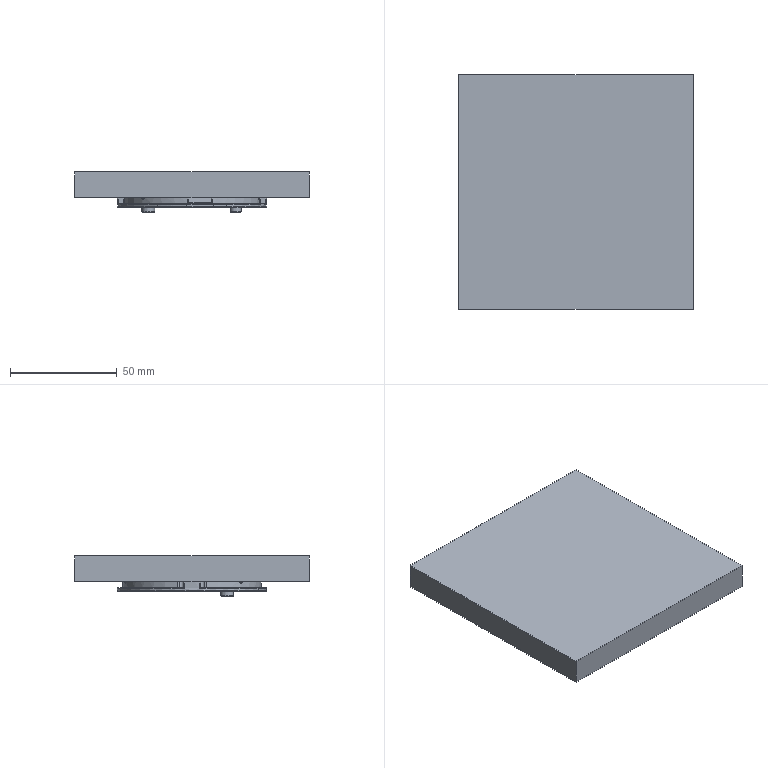NC program | NX | posted with a generic post | part box 110 x 110 x 18.8 mm
Lines 7252 to 9086 of 9447, first 1548 of 1823 lines:
(CAVITY_MILL_COPY_1_COPY_COPY , TOOL : D2)
N14466 T02 M6
N14468 G54
N14470 G17 G0 G90 X19.668 Y-21.389 S9500 M3
N14472 G43 Z30. H2
N14474 Z-4.143
N14476 G94 G1 Z-5.143 F1000.
N14478 X20.63 Y-20.963
N14480 G3 X20.925 Y-20.56 R0.5
N14482 X20.616 Y-20. R0.557
N14484 G1 X20.071
N14486 G3 X19.271 Y-20.4 R1.
N14488 G1 Z-4.143
N14490 G0 Z30.
N14492 X14.4 Y-21.675
N14494 Z-10.625
N14496 G1 Z-11.625
N14498 G3 X14.825 Y-20.857 R1.
N14500 G1 Y-20.
N14502 X13.968
N14504 G3 X13.168 Y-20.4 R1.
N14506 G1 Z-10.625
N14508 G0 X14.325 Y-21.675 Z-10.75
N14510 G1 Z-11.75
N14512 G3 X14.75 Y-20.857 R1.
N14514 G1 Y-20.
N14516 X13.893
N14518 G3 X13.093 Y-20.4 R1.
N14520 G1 Z-10.75
N14522 G0 X14.325 Y-21.675 Z-10.875
N14524 G1 Z-11.875
N14526 G3 X14.75 Y-20.857 R1.
N14528 G1 Y-20.
N14530 X13.893
N14532 G3 X13.093 Y-20.4 R1.
N14534 G1 Z-10.875
N14536 G0 X14.325 Y-21.675 Z-11.
N14538 G1 Z-12.
N14540 G3 X14.75 Y-20.857 R1.
N14542 G1 Y-20.
N14544 X13.893
N14546 G3 X13.093 Y-20.4 R1.
N14548 G1 Z-11.
N14550 G0 Z30.
N14552 X24.9 Y-13.399
N14554 Z-4.143
N14556 G1 Z-5.143
N14558 G3 X24.5 Y-14.199 R1.
N14560 G1 Y-14.744
N14562 G3 X25.06 Y-15.053 R0.557
N14564 X25.463 Y-14.758 R0.5
N14566 G1 X25.301 Y-14.289
N14568 Z-4.143
N14570 G0 Z30.
N14572 X33.412 Y-4.088
N14574 Z-4.143
N14576 G1 Z-5.143
N14578 G3 X32.74 Y-4.451 R1.
N14580 G2 X32.126 Y-4.949 R1.943
N14582 G1 X32.092 Y-4.97
N14584 X32.086 Y-5.011
N14586 X32.112 Y-5.04
N14588 G2 X32.545 Y-5.702 R1.943
N14590 G3 X33.075 Y-6.251 R1.
N14592 G1 Z-4.143
N14594 G0 X33.471 Y-4.092 Z-4.286
N14596 G1 Z-5.286
N14598 G3 X32.802 Y-4.465 R1.
N14600 G2 X32.18 Y-4.986 R2.
N14602 G1 X32.152 Y-5.
N14604 G2 X32.609 Y-5.708 R2.
N14606 G3 X33.133 Y-6.266 R1.
N14608 G1 Z-4.286
N14610 G0 X33.471 Y-4.092 Z-4.429
N14612 G1 Z-5.429
N14614 G3 X32.802 Y-4.465 R1.
N14616 G2 X32.18 Y-4.986 R2.
N14618 G1 X32.152 Y-5.
N14620 G2 X32.609 Y-5.708 R2.
N14622 G3 X33.133 Y-6.266 R1.
N14624 G1 Z-4.429
N14626 G0 X33.471 Y-4.092 Z-4.571
N14628 G1 Z-5.571
N14630 G3 X32.802 Y-4.465 R1.
N14632 G2 X32.18 Y-4.986 R2.
N14634 G1 X32.152 Y-5.
N14636 G2 X32.609 Y-5.708 R2.
N14638 G3 X33.133 Y-6.266 R1.
N14640 G1 Z-4.571
N14642 G0 X33.471 Y-4.092 Z-4.714
N14644 G1 Z-5.714
N14646 G3 X32.802 Y-4.465 R1.
N14648 G2 X32.18 Y-4.986 R2.
N14650 G1 X32.152 Y-5.
N14652 G2 X32.609 Y-5.708 R2.
N14654 G3 X33.133 Y-6.266 R1.
N14656 G1 Z-4.714
N14658 G0 X33.471 Y-4.092 Z-4.857
N14660 G1 Z-5.857
N14662 G3 X32.802 Y-4.465 R1.
N14664 G2 X32.18 Y-4.986 R2.
N14666 G1 X32.152 Y-5.
N14668 G2 X32.609 Y-5.708 R2.
N14670 G3 X33.133 Y-6.266 R1.
N14672 G1 Z-4.857
N14674 G0 X33.471 Y-4.092 Z-5.
N14676 G1 Z-6.
N14678 G3 X32.802 Y-4.465 R1.
N14680 G2 X32.18 Y-4.986 R2.
N14682 G1 X32.152 Y-5.
N14684 G2 X32.609 Y-5.708 R2.
N14686 G3 X33.133 Y-6.266 R1.
N14688 G1 Z-5.
N14690 G0 X33.471 Y-4.092 Z-5.15
N14692 G1 Z-6.15
N14694 G3 X32.802 Y-4.465 R1.
N14696 G2 X32.18 Y-4.986 R2.
N14698 G1 X32.152 Y-5.
N14700 G2 X32.609 Y-5.708 R2.
N14702 G3 X33.133 Y-6.266 R1.
N14704 G1 Z-5.15
N14706 G0 X33.471 Y-4.092 Z-5.3
N14708 G1 Z-6.3
N14710 G3 X32.802 Y-4.465 R1.
N14712 G2 X32.18 Y-4.986 R2.
N14714 G1 X32.152 Y-5.
N14716 G2 X32.609 Y-5.708 R2.
N14718 G3 X33.133 Y-6.266 R1.
N14720 G1 Z-5.3
N14722 G0 X33.471 Y-4.092 Z-5.45
N14724 G1 Z-6.45
N14726 G3 X32.802 Y-4.465 R1.
N14728 G2 X32.18 Y-4.986 R2.
N14730 G1 X32.152 Y-5.
N14732 G2 X32.609 Y-5.708 R2.
N14734 G3 X33.133 Y-6.266 R1.
N14736 G1 Z-5.45
N14738 G0 X33.471 Y-4.092 Z-5.6
N14740 G1 Z-6.6
N14742 G3 X32.802 Y-4.465 R1.
N14744 G2 X32.18 Y-4.986 R2.
N14746 G1 X32.152 Y-5.
N14748 G2 X32.609 Y-5.708 R2.
N14750 G3 X33.133 Y-6.266 R1.
N14752 G1 Z-5.6
N14754 G0 X33.471 Y-4.092 Z-5.75
N14756 G1 Z-6.75
N14758 G3 X32.802 Y-4.465 R1.
N14760 G2 X32.18 Y-4.986 R2.
N14762 G1 X32.152 Y-5.
N14764 G2 X32.609 Y-5.708 R2.
N14766 G3 X33.133 Y-6.266 R1.
N14768 G1 Z-5.75
N14770 G0 X33.471 Y-4.092 Z-5.9
N14772 G1 Z-6.9
N14774 G3 X32.802 Y-4.465 R1.
N14776 G2 X32.18 Y-4.986 R2.
N14778 G1 X32.152 Y-5.
N14780 G2 X32.609 Y-5.708 R2.
N14782 G3 X33.133 Y-6.266 R1.
N14784 G1 Z-5.9
N14786 G0 X33.471 Y-4.092 Z-6.05
N14788 G1 Z-7.05
N14790 G3 X32.802 Y-4.465 R1.
N14792 G2 X32.18 Y-4.986 R2.
N14794 G1 X32.152 Y-5.
N14796 G2 X32.609 Y-5.708 R2.
N14798 G3 X33.133 Y-6.266 R1.
N14800 G1 Z-6.05
N14802 G0 X33.471 Y-4.092 Z-6.2
N14804 G1 Z-7.2
N14806 G3 X32.802 Y-4.465 R1.
N14808 G2 X32.18 Y-4.986 R2.
N14810 G1 X32.152 Y-5.
N14812 G2 X32.609 Y-5.708 R2.
N14814 G3 X33.133 Y-6.266 R1.
N14816 G1 Z-6.2
N14818 G0 X33.471 Y-4.092 Z-6.35
N14820 G1 Z-7.35
N14822 G3 X32.802 Y-4.465 R1.
N14824 G2 X32.18 Y-4.986 R2.
N14826 G1 X32.152 Y-5.
N14828 G2 X32.609 Y-5.708 R2.
N14830 G3 X33.133 Y-6.266 R1.
N14832 G1 Z-6.35
N14834 G0 X33.471 Y-4.092 Z-6.5
N14836 G1 Z-7.5
N14838 G3 X32.802 Y-4.465 R1.
N14840 G2 X32.18 Y-4.986 R2.
N14842 G1 X32.152 Y-5.
N14844 G2 X32.609 Y-5.708 R2.
N14846 G3 X33.133 Y-6.266 R1.
N14848 G1 Z-6.5
N14850 G0 X33.471 Y-4.092 Z-6.65
N14852 G1 Z-7.65
N14854 G3 X32.802 Y-4.465 R1.
N14856 G2 X32.18 Y-4.986 R2.
N14858 G1 X32.152 Y-5.
N14860 G2 X32.609 Y-5.708 R2.
N14862 G3 X33.133 Y-6.266 R1.
N14864 G1 Z-6.65
N14866 G0 X33.471 Y-4.092 Z-6.8
N14868 G1 Z-7.8
N14870 G3 X32.802 Y-4.465 R1.
N14872 G2 X32.18 Y-4.986 R2.
N14874 G1 X32.152 Y-5.
N14876 G2 X32.609 Y-5.708 R2.
N14878 G3 X33.133 Y-6.266 R1.
N14880 G1 Z-6.8
N14882 G0 X33.471 Y-4.092 Z-6.95
N14884 G1 Z-7.95
N14886 G3 X32.802 Y-4.465 R1.
N14888 G2 X32.18 Y-4.986 R2.
N14890 G1 X32.152 Y-5.
N14892 G2 X32.609 Y-5.708 R2.
N14894 G3 X33.133 Y-6.266 R1.
N14896 G1 Z-6.95
N14898 G0 X33.471 Y-4.092 Z-7.1
N14900 G1 Z-8.1
N14902 G3 X32.802 Y-4.465 R1.
N14904 G2 X32.18 Y-4.986 R2.
N14906 G1 X32.152 Y-5.
N14908 G2 X32.609 Y-5.708 R2.
N14910 G3 X33.133 Y-6.266 R1.
N14912 G1 Z-7.1
N14914 G0 X33.471 Y-4.092 Z-7.25
N14916 G1 Z-8.25
N14918 G3 X32.802 Y-4.465 R1.
N14920 G2 X32.188 Y-4.981 R2.
N14922 G1 X32.152 Y-5.
N14924 G2 X32.609 Y-5.708 R2.
N14926 G3 X33.133 Y-6.266 R1.
N14928 G1 Z-7.25
N14930 G0 X33.471 Y-4.092 Z-7.4
N14932 G1 Z-8.4
N14934 G3 X32.802 Y-4.465 R1.
N14936 G2 X32.188 Y-4.981 R2.
N14938 G1 X32.152 Y-5.
N14940 G2 X32.609 Y-5.708 R2.
N14942 G3 X33.133 Y-6.266 R1.
N14944 G1 Z-7.4
N14946 G0 X33.471 Y-4.092 Z-7.55
N14948 G1 Z-8.55
N14950 G3 X32.802 Y-4.465 R1.
N14952 G2 X32.188 Y-4.981 R2.
N14954 G1 X32.152 Y-5.
N14956 G2 X32.609 Y-5.708 R2.
N14958 G3 X33.133 Y-6.266 R1.
N14960 G1 Z-7.55
N14962 G0 X33.471 Y-4.092 Z-7.7
N14964 G1 Z-8.7
N14966 G3 X32.802 Y-4.465 R1.
N14968 G2 X32.188 Y-4.981 R2.
N14970 G1 X32.152 Y-5.
N14972 G2 X32.609 Y-5.708 R2.
N14974 G3 X33.133 Y-6.266 R1.
N14976 G1 Z-7.7
N14978 G0 X33.471 Y-4.092 Z-7.85
N14980 G1 Z-8.85
N14982 G3 X32.802 Y-4.465 R1.
N14984 G2 X32.188 Y-4.981 R2.
N14986 G1 X32.152 Y-5.
N14988 G2 X32.609 Y-5.708 R2.
N14990 G3 X33.133 Y-6.266 R1.
N14992 G1 Z-7.85
N14994 G0 X33.471 Y-4.092 Z-8.
N14996 G1 Z-9.
N14998 G3 X32.802 Y-4.465 R1.
N15000 G2 X32.188 Y-4.981 R2.
N15002 G1 X32.152 Y-5.
N15004 G2 X32.609 Y-5.708 R2.
N15006 G3 X33.133 Y-6.266 R1.
N15008 G1 Z-8.
N15010 G0 X34.2 Y-5.347 Z-8.147
N15012 G1 Z-9.147
N15014 G3 X33.4 Y-4.947 R1.
N15016 G1 X32.248
N15018 X32.188 Y-4.981
N15020 X32.152 Y-5.
N15022 G2 X32.694 Y-5.996 R2.
N15024 G3 X33.128 Y-6.627 R1.
N15026 G1 Z-8.147
N15028 G0 X34.222 Y-5.4 Z-8.294
N15030 G1 Z-9.294
N15032 G3 X33.422 Y-5. R1.
N15034 G1 X32.198
N15036 X32.152
N15038 G2 X32.703 Y-6.041 R2.
N15040 G3 X33.123 Y-6.682 R1.
N15042 G1 Z-8.294
N15044 G0 X34.222 Y-5.4 Z-8.441
N15046 G1 Z-9.441
N15048 G3 X33.422 Y-5. R1.
N15050 G1 X32.198
N15052 X32.152
N15054 G2 X32.703 Y-6.041 R2.
N15056 G3 X33.123 Y-6.682 R1.
N15058 G1 Z-8.441
N15060 G0 X34.222 Y-5.4 Z-8.588
N15062 G1 Z-9.588
N15064 G3 X33.422 Y-5. R1.
N15066 G1 X32.198
N15068 X32.152
N15070 G2 X32.703 Y-6.041 R2.
N15072 G3 X33.123 Y-6.682 R1.
N15074 G1 Z-8.588
N15076 G0 X34.222 Y-5.4 Z-8.735
N15078 G1 Z-9.735
N15080 G3 X33.422 Y-5. R1.
N15082 G1 X32.198
N15084 X32.152
N15086 G2 X32.703 Y-6.041 R2.
N15088 G3 X33.123 Y-6.682 R1.
N15090 G1 Z-8.735
N15092 G0 X34.222 Y-5.4 Z-8.882
N15094 G1 Z-9.882
N15096 G3 X33.422 Y-5. R1.
N15098 G1 X32.198
N15100 X32.152
N15102 G2 X32.703 Y-6.041 R2.
N15104 G3 X33.123 Y-6.682 R1.
N15106 G1 Z-8.882
N15108 G0 X34.222 Y-5.4 Z-9.029
N15110 G1 Z-10.029
N15112 G3 X33.422 Y-5. R1.
N15114 G1 X32.198
N15116 X32.152
N15118 G2 X32.703 Y-6.041 R2.
N15120 G3 X33.123 Y-6.682 R1.
N15122 G1 Z-9.029
N15124 G0 X34.222 Y-5.4 Z-9.176
N15126 G1 Z-10.176
N15128 G3 X33.422 Y-5. R1.
N15130 G1 X32.198
N15132 X32.152
N15134 G2 X32.703 Y-6.041 R2.
N15136 G3 X33.123 Y-6.682 R1.
N15138 G1 Z-9.176
N15140 G0 X34.222 Y-5.4 Z-9.324
N15142 G1 Z-10.324
N15144 G3 X33.422 Y-5. R1.
N15146 G1 X32.198
N15148 X32.152
N15150 G2 X32.703 Y-6.041 R2.
N15152 G3 X33.123 Y-6.682 R1.
N15154 G1 Z-9.324
N15156 G0 X34.222 Y-5.4 Z-9.471
N15158 G1 Z-10.471
N15160 G3 X33.422 Y-5. R1.
N15162 G1 X32.198
N15164 X32.152
N15166 G2 X32.703 Y-6.041 R2.
N15168 G3 X33.123 Y-6.682 R1.
N15170 G1 Z-9.471
N15172 G0 X34.222 Y-5.4 Z-9.618
N15174 G1 Z-10.618
N15176 G3 X33.422 Y-5. R1.
N15178 G1 X32.198
N15180 X32.152
N15182 G2 X32.703 Y-6.041 R2.
N15184 G3 X33.123 Y-6.682 R1.
N15186 G1 Z-9.618
N15188 G0 X34.222 Y-5.4 Z-9.765
N15190 G1 Z-10.765
N15192 G3 X33.422 Y-5. R1.
N15194 G1 X32.198
N15196 X32.152
N15198 G2 X32.703 Y-6.041 R2.
N15200 G3 X33.123 Y-6.682 R1.
N15202 G1 Z-9.765
N15204 G0 X34.222 Y-5.4 Z-9.912
N15206 G1 Z-10.912
N15208 G3 X33.422 Y-5. R1.
N15210 G1 X32.198
N15212 X32.152
N15214 G2 X32.703 Y-6.041 R2.
N15216 G3 X33.123 Y-6.682 R1.
N15218 G1 Z-9.912
N15220 G0 X34.222 Y-5.4 Z-10.059
N15222 G1 Z-11.059
N15224 G3 X33.422 Y-5. R1.
N15226 G1 X32.198
N15228 X32.152
N15230 G2 X32.703 Y-6.041 R2.
N15232 G3 X33.123 Y-6.682 R1.
N15234 G1 Z-10.059
N15236 G0 X34.222 Y-5.4 Z-10.206
N15238 G1 Z-11.206
N15240 G3 X33.422 Y-5. R1.
N15242 G1 X32.198
N15244 X32.152
N15246 G2 X32.703 Y-6.041 R2.
N15248 G3 X33.123 Y-6.682 R1.
N15250 G1 Z-10.206
N15252 G0 X34.222 Y-5.4 Z-10.353
N15254 G1 Z-11.353
N15256 G3 X33.422 Y-5. R1.
N15258 G1 X32.187
N15260 X32.152
N15262 G2 X32.703 Y-6.041 R2.
N15264 G3 X33.123 Y-6.682 R1.
N15266 G1 Z-10.353
N15268 G0 X34.222 Y-5.4 Z-10.5
N15270 G1 Z-11.5
N15272 G3 X33.422 Y-5. R1.
N15274 G1 X32.187
N15276 X32.152
N15278 G2 X32.703 Y-6.041 R2.
N15280 G3 X33.123 Y-6.682 R1.
N15282 G1 Z-10.5
N15284 G0 X34.222 Y-5.4 Z-10.625
N15286 G1 Z-11.625
N15288 G3 X33.422 Y-5. R1.
N15290 G1 X32.187
N15292 X32.152
N15294 G2 X32.703 Y-6.041 R2.
N15296 G3 X33.123 Y-6.682 R1.
N15298 G1 Z-10.625
N15300 G0 X34.222 Y-5.4 Z-10.75
N15302 G1 Z-11.75
N15304 G3 X33.422 Y-5. R1.
N15306 G1 X32.187
N15308 X32.152
N15310 G2 X32.703 Y-6.041 R2.
N15312 G3 X33.123 Y-6.682 R1.
N15314 G1 Z-10.75
N15316 G0 X34.222 Y-5.4 Z-10.875
N15318 G1 Z-11.875
N15320 G3 X33.422 Y-5. R1.
N15322 G1 X32.187
N15324 X32.152
N15326 G2 X32.703 Y-6.041 R2.
N15328 G3 X33.123 Y-6.682 R1.
N15330 G1 Z-10.875
N15332 G0 X34.222 Y-5.4 Z-11.
N15334 G1 Z-12.
N15336 G3 X33.422 Y-5. R1.
N15338 G1 X32.187
N15340 X32.152
N15342 G2 X32.703 Y-6.041 R2.
N15344 G3 X33.123 Y-6.682 R1.
N15346 G1 Z-11.
N15348 G0 Z30.
N15350 X33.075 Y6.251
N15352 Z-4.143
N15354 G1 Z-5.143
N15356 G3 X32.545 Y5.702 R1.
N15358 G2 X32.112 Y5.04 R1.943
N15360 G1 X32.086 Y5.011
N15362 X32.092 Y4.97
N15364 X32.126 Y4.949
N15366 G2 X32.74 Y4.451 R1.943
N15368 G3 X33.412 Y4.088 R1.
N15370 G1 Z-4.143
N15372 G0 X33.133 Y6.266 Z-4.286
N15374 G1 Z-5.286
N15376 G3 X32.609 Y5.708 R1.
N15378 G2 X32.152 Y5. R2.
N15380 X32.802 Y4.465 R2.
N15382 G3 X33.471 Y4.092 R1.
N15384 G1 Z-4.286
N15386 G0 X33.133 Y6.266 Z-4.429
N15388 G1 Z-5.429
N15390 G3 X32.609 Y5.708 R1.
N15392 G2 X32.152 Y5. R2.
N15394 X32.802 Y4.464 R2.
N15396 G3 X33.471 Y4.092 R1.
N15398 G1 Z-4.429
N15400 G0 X33.133 Y6.266 Z-4.571
N15402 G1 Z-5.571
N15404 G3 X32.609 Y5.708 R1.
N15406 G2 X32.152 Y5. R2.
N15408 X32.802 Y4.464 R2.
N15410 G3 X33.471 Y4.092 R1.
N15412 G1 Z-4.571
N15414 G0 X33.133 Y6.266 Z-4.714
N15416 G1 Z-5.714
N15418 G3 X32.609 Y5.708 R1.
N15420 G2 X32.152 Y5. R2.
N15422 X32.802 Y4.464 R2.
N15424 G3 X33.471 Y4.092 R1.
N15426 G1 Z-4.714
N15428 G0 X33.133 Y6.266 Z-4.857
N15430 G1 Z-5.857
N15432 G3 X32.609 Y5.708 R1.
N15434 G2 X32.152 Y5. R2.
N15436 X32.802 Y4.465 R2.
N15438 G3 X33.471 Y4.092 R1.
N15440 G1 Z-4.857
N15442 G0 X33.133 Y6.266 Z-5.
N15444 G1 Z-6.
N15446 G3 X32.609 Y5.708 R1.
N15448 G2 X32.152 Y5. R2.
N15450 X32.802 Y4.465 R2.
N15452 G3 X33.471 Y4.092 R1.
N15454 G1 Z-5.
N15456 G0 X33.133 Y6.266 Z-5.15
N15458 G1 Z-6.15
N15460 G3 X32.609 Y5.708 R1.
N15462 G2 X32.152 Y5. R2.
N15464 X32.802 Y4.465 R2.
N15466 G3 X33.471 Y4.092 R1.
N15468 G1 Z-5.15
N15470 G0 X33.133 Y6.266 Z-5.3
N15472 G1 Z-6.3
N15474 G3 X32.609 Y5.708 R1.
N15476 G2 X32.152 Y5. R2.
N15478 X32.802 Y4.465 R2.
N15480 G3 X33.471 Y4.092 R1.
N15482 G1 Z-5.3
N15484 G0 X33.133 Y6.266 Z-5.45
N15486 G1 Z-6.45
N15488 G3 X32.609 Y5.708 R1.
N15490 G2 X32.152 Y5. R2.
N15492 X32.802 Y4.465 R2.
N15494 G3 X33.471 Y4.092 R1.
N15496 G1 Z-5.45
N15498 G0 X33.133 Y6.266 Z-5.6
N15500 G1 Z-6.6
N15502 G3 X32.609 Y5.708 R1.
N15504 G2 X32.152 Y5. R2.
N15506 X32.802 Y4.465 R2.
N15508 G3 X33.471 Y4.092 R1.
N15510 G1 Z-5.6
N15512 G0 X33.133 Y6.266 Z-5.75
N15514 G1 Z-6.75
N15516 G3 X32.609 Y5.708 R1.
N15518 G2 X32.152 Y5. R2.
N15520 X32.802 Y4.465 R2.
N15522 G3 X33.471 Y4.092 R1.
N15524 G1 Z-5.75
N15526 G0 X33.133 Y6.266 Z-5.9
N15528 G1 Z-6.9
N15530 G3 X32.609 Y5.708 R1.
N15532 G2 X32.152 Y5. R2.
N15534 X32.802 Y4.464 R2.
N15536 G3 X33.471 Y4.092 R1.
N15538 G1 Z-5.9
N15540 G0 X33.133 Y6.266 Z-6.05
N15542 G1 Z-7.05
N15544 G3 X32.609 Y5.708 R1.
N15546 G2 X32.152 Y5. R2.
N15548 X32.802 Y4.464 R2.
N15550 G3 X33.471 Y4.092 R1.
N15552 G1 Z-6.05
N15554 G0 X33.133 Y6.266 Z-6.2
N15556 G1 Z-7.2
N15558 G3 X32.609 Y5.708 R1.
N15560 G2 X32.152 Y5. R2.
N15562 X32.802 Y4.464 R2.
N15564 G3 X33.471 Y4.092 R1.
N15566 G1 Z-6.2
N15568 G0 X33.133 Y6.266 Z-6.35
N15570 G1 Z-7.35
N15572 G3 X32.609 Y5.708 R1.
N15574 G2 X32.152 Y5. R2.
N15576 X32.802 Y4.464 R2.
N15578 G3 X33.471 Y4.092 R1.
N15580 G1 Z-6.35
N15582 G0 X33.133 Y6.266 Z-6.5
N15584 G1 Z-7.5
N15586 G3 X32.609 Y5.708 R1.
N15588 G2 X32.152 Y5. R2.
N15590 X32.802 Y4.464 R2.
N15592 G3 X33.471 Y4.092 R1.
N15594 G1 Z-6.5
N15596 G0 X33.133 Y6.266 Z-6.65
N15598 G1 Z-7.65
N15600 G3 X32.609 Y5.708 R1.
N15602 G2 X32.152 Y5. R2.
N15604 X32.802 Y4.464 R2.
N15606 G3 X33.471 Y4.092 R1.
N15608 G1 Z-6.65
N15610 G0 X33.133 Y6.266 Z-6.8
N15612 G1 Z-7.8
N15614 G3 X32.609 Y5.708 R1.
N15616 G2 X32.152 Y5. R2.
N15618 X32.802 Y4.464 R2.
N15620 G3 X33.471 Y4.092 R1.
N15622 G1 Z-6.8
N15624 G0 X33.133 Y6.266 Z-6.95
N15626 G1 Z-7.95
N15628 G3 X32.609 Y5.708 R1.
N15630 G2 X32.152 Y5. R2.
N15632 X32.802 Y4.464 R2.
N15634 G3 X33.471 Y4.092 R1.
N15636 G1 Z-6.95
N15638 G0 X33.133 Y6.266 Z-7.1
N15640 G1 Z-8.1
N15642 G3 X32.609 Y5.708 R1.
N15644 G2 X32.152 Y5. R2.
N15646 X32.802 Y4.464 R2.
N15648 G3 X33.471 Y4.092 R1.
N15650 G1 Z-7.1
N15652 G0 X33.133 Y6.266 Z-7.25
N15654 G1 Z-8.25
N15656 G3 X32.609 Y5.708 R1.
N15658 G2 X32.152 Y5. R2.
N15660 X32.802 Y4.464 R2.
N15662 G3 X33.471 Y4.092 R1.
N15664 G1 Z-7.25
N15666 G0 X33.133 Y6.266 Z-7.4
N15668 G1 Z-8.4
N15670 G3 X32.609 Y5.708 R1.
N15672 G2 X32.152 Y5. R2.
N15674 X32.802 Y4.464 R2.
N15676 G3 X33.471 Y4.092 R1.
N15678 G1 Z-7.4
N15680 G0 X33.133 Y6.266 Z-7.55
N15682 G1 Z-8.55
N15684 G3 X32.609 Y5.708 R1.
N15686 G2 X32.152 Y5. R2.
N15688 X32.802 Y4.464 R2.
N15690 G3 X33.471 Y4.092 R1.
N15692 G1 Z-7.55
N15694 G0 X33.133 Y6.266 Z-7.7
N15696 G1 Z-8.7
N15698 G3 X32.609 Y5.708 R1.
N15700 G2 X32.152 Y5. R2.
N15702 X32.802 Y4.464 R2.
N15704 G3 X33.471 Y4.092 R1.
N15706 G1 Z-7.7
N15708 G0 X33.133 Y6.266 Z-7.85
N15710 G1 Z-8.85
N15712 G3 X32.609 Y5.708 R1.
N15714 G2 X32.152 Y5. R2.
N15716 X32.802 Y4.464 R2.
N15718 G3 X33.471 Y4.092 R1.
N15720 G1 Z-7.85
N15722 G0 X33.133 Y6.266 Z-8.
N15724 G1 Z-9.
N15726 G3 X32.609 Y5.708 R1.
N15728 G2 X32.152 Y5. R2.
N15730 X32.802 Y4.464 R2.
N15732 G3 X33.471 Y4.092 R1.
N15734 G1 Z-8.
N15736 G0 X33.128 Y6.627 Z-8.147
N15738 G1 Z-9.147
N15740 G3 X32.694 Y5.996 R1.
N15742 G2 X32.152 Y5. R2.
N15744 G1 X32.248 Y4.947
N15746 X33.4
N15748 G3 X34.2 Y5.347 R1.
N15750 G1 Z-8.147
N15752 G0 X33.123 Y6.682 Z-8.294
N15754 G1 Z-9.294
N15756 G3 X32.703 Y6.041 R1.
N15758 G2 X32.152 Y5. R2.
N15760 G1 X32.155 Y4.999
N15762 X32.211 Y5.
N15764 X33.422
N15766 G3 X34.222 Y5.4 R1.
N15768 G1 Z-8.294
N15770 G0 X33.123 Y6.682 Z-8.441
N15772 G1 Z-9.441
N15774 G3 X32.703 Y6.041 R1.
N15776 G2 X32.152 Y5. R2.
N15778 G1 X32.154 Y4.999
N15780 X32.211 Y5.
N15782 X33.422
N15784 G3 X34.222 Y5.4 R1.
N15786 G1 Z-8.441
N15788 G0 X33.123 Y6.682 Z-8.588
N15790 G1 Z-9.588
N15792 G3 X32.703 Y6.041 R1.
N15794 G2 X32.152 Y5. R2.
N15796 G1 X32.154 Y4.999
N15798 X32.211 Y5.
N15800 X33.422
N15802 G3 X34.222 Y5.4 R1.
N15804 G1 Z-8.588
N15806 G0 X33.123 Y6.682 Z-8.735
N15808 G1 Z-9.735
N15810 G3 X32.703 Y6.041 R1.
N15812 G2 X32.152 Y5. R2.
N15814 G1 X33.422
N15816 G3 X34.222 Y5.4 R1.
N15818 G1 Z-8.735
N15820 G0 X33.123 Y6.682 Z-8.882
N15822 G1 Z-9.882
N15824 G3 X32.703 Y6.041 R1.
N15826 G2 X32.152 Y5. R2.
N15828 G1 X33.422
N15830 G3 X34.222 Y5.4 R1.
N15832 G1 Z-8.882
N15834 G0 X33.123 Y6.682 Z-9.029
N15836 G1 Z-10.029
N15838 G3 X32.703 Y6.041 R1.
N15840 G2 X32.152 Y5. R2.
N15842 G1 X33.422
N15844 G3 X34.222 Y5.4 R1.
N15846 G1 Z-9.029
N15848 G0 X33.123 Y6.682 Z-9.176
N15850 G1 Z-10.176
N15852 G3 X32.703 Y6.041 R1.
N15854 G2 X32.152 Y5. R2.
N15856 G1 X33.422
N15858 G3 X34.222 Y5.4 R1.
N15860 G1 Z-9.176
N15862 G0 X33.123 Y6.682 Z-9.324
N15864 G1 Z-10.324
N15866 G3 X32.703 Y6.041 R1.
N15868 G2 X32.152 Y5. R2.
N15870 G1 X33.422
N15872 G3 X34.222 Y5.4 R1.
N15874 G1 Z-9.324
N15876 G0 X33.123 Y6.682 Z-9.471
N15878 G1 Z-10.471
N15880 G3 X32.703 Y6.041 R1.
N15882 G2 X32.152 Y5. R2.
N15884 G1 X33.422
N15886 G3 X34.222 Y5.4 R1.
N15888 G1 Z-9.471
N15890 G0 X33.123 Y6.682 Z-9.618
N15892 G1 Z-10.618
N15894 G3 X32.703 Y6.041 R1.
N15896 G2 X32.153 Y5. R2.001
N15898 G1 X32.211
N15900 X33.422
N15902 G3 X34.222 Y5.4 R1.
N15904 G1 Z-9.618
N15906 G0 X33.123 Y6.682 Z-9.765
N15908 G1 Z-10.765
N15910 G3 X32.703 Y6.041 R1.
N15912 G2 X32.153 Y5. R2.001
N15914 G1 X32.211
N15916 X33.422
N15918 G3 X34.222 Y5.4 R1.
N15920 G1 Z-9.765
N15922 G0 X33.123 Y6.682 Z-9.912
N15924 G1 Z-10.912
N15926 G3 X32.703 Y6.041 R1.
N15928 G2 X32.153 Y5. R2.
N15930 G1 X32.211
N15932 X33.422
N15934 G3 X34.222 Y5.4 R1.
N15936 G1 Z-9.912
N15938 G0 X33.123 Y6.682 Z-10.059
N15940 G1 Z-11.059
N15942 G3 X32.703 Y6.041 R1.
N15944 G2 X32.152 Y5. R2.
N15946 G1 X32.211
N15948 X33.422
N15950 G3 X34.222 Y5.4 R1.
N15952 G1 Z-10.059
N15954 G0 X33.123 Y6.682 Z-10.206
N15956 G1 Z-11.206
N15958 G3 X32.703 Y6.041 R1.
N15960 G2 X32.152 Y5. R2.
N15962 G1 X32.211
N15964 X33.422
N15966 G3 X34.222 Y5.4 R1.
N15968 G1 Z-10.206
N15970 G0 X33.123 Y6.682 Z-10.353
N15972 G1 Z-11.353
N15974 G3 X32.703 Y6.041 R1.
N15976 G2 X32.152 Y5. R2.
N15978 G1 X32.187
N15980 X33.422
N15982 G3 X34.222 Y5.4 R1.
N15984 G1 Z-10.353
N15986 G0 X33.123 Y6.682 Z-10.5
N15988 G1 Z-11.5
N15990 G3 X32.703 Y6.041 R1.
N15992 G2 X32.152 Y5. R2.
N15994 G1 X32.187
N15996 X33.422
N15998 G3 X34.222 Y5.4 R1.
N16000 G1 Z-10.5
N16002 G0 X33.123 Y6.682 Z-10.625
N16004 G1 Z-11.625
N16006 G3 X32.703 Y6.041 R1.
N16008 G2 X32.152 Y5. R2.
N16010 G1 X32.187
N16012 X33.422
N16014 G3 X34.222 Y5.4 R1.
N16016 G1 Z-10.625
N16018 G0 X33.123 Y6.682 Z-10.75
N16020 G1 Z-11.75
N16022 G3 X32.703 Y6.041 R1.
N16024 G2 X32.152 Y5. R2.
N16026 G1 X32.187
N16028 X33.422
N16030 G3 X34.222 Y5.4 R1.
N16032 G1 Z-10.75
N16034 G0 X33.123 Y6.682 Z-10.875
N16036 G1 Z-11.875
N16038 G3 X32.703 Y6.041 R1.
N16040 G2 X32.152 Y5. R2.
N16042 G1 X32.187
N16044 X33.422
N16046 G3 X34.222 Y5.4 R1.
N16048 G1 Z-10.875
N16050 G0 X33.123 Y6.682 Z-11.
N16052 G1 Z-12.
N16054 G3 X32.703 Y6.041 R1.
N16056 G2 X32.152 Y5. R2.
N16058 G1 X32.187
N16060 X33.422
N16062 G3 X34.222 Y5.4 R1.
N16064 G1 Z-11.
N16066 G0 Z30.
N16068 X25.301 Y14.289
N16070 Z-4.143
N16072 G1 Z-5.143
N16074 X25.463 Y14.758
N16076 G3 X25.06 Y15.053 R0.5
N16078 X24.5 Y14.744 R0.557
N16080 G1 Y14.199
N16082 G3 X24.9 Y13.399 R1.
N16084 G1 Z-4.143
N16086 G0 Z30.
N16088 X19.271 Y20.4
N16090 Z-4.143
N16092 G1 Z-5.143
N16094 G3 X20.071 Y20. R1.
N16096 G1 X20.616
N16098 G3 X20.925 Y20.56 R0.557
N16100 X20.63 Y20.963 R0.5
N16102 G1 X19.668 Y21.389
N16104 Z-4.143
N16106 G0 Z30.
N16108 X8.1 Y-9.332
N16110 Z-10.625
N16112 G1 Z-11.625
N16114 G3 X8.5 Y-8.532 R1.
N16116 G1 Y-7.675
N16118 X7.643
N16120 G3 X6.843 Y-8.075 R1.
N16122 G1 Z-10.625
N16124 G0 X8.1 Y-9.407 Z-10.75
N16126 G1 Z-11.75
N16128 G3 X8.5 Y-8.607 R1.
N16130 G1 Y-7.75
N16132 X7.643
N16134 G3 X6.843 Y-8.15 R1.
N16136 G1 Z-10.75
N16138 G0 X8.1 Y-9.407 Z-10.875
N16140 G1 Z-11.875
N16142 G3 X8.5 Y-8.607 R1.
N16144 G1 Y-7.75
N16146 X7.643
N16148 G3 X6.843 Y-8.15 R1.
N16150 G1 Z-10.875
N16152 G0 X8.1 Y-9.407 Z-11.
N16154 G1 Z-12.
N16156 G3 X8.5 Y-8.607 R1.
N16158 G1 Y-7.75
N16160 X7.643
N16162 G3 X6.843 Y-8.15 R1.
N16164 G1 Z-11.
N16166 G0 Z30.
N16168 X-33.412 Y4.088
N16170 Z-4.143
N16172 G1 Z-5.143
N16174 G3 X-32.74 Y4.451 R1.
N16176 G2 X-32.126 Y4.949 R1.943
N16178 G1 X-32.092 Y4.97
N16180 X-32.086 Y5.011
N16182 X-32.112 Y5.04
N16184 G2 X-32.545 Y5.702 R1.943
N16186 G3 X-33.075 Y6.251 R1.
N16188 G1 Z-4.143
N16190 G0 X-33.471 Y4.092 Z-4.286
N16192 G1 Z-5.286
N16194 G3 X-32.802 Y4.465 R1.
N16196 G2 X-32.152 Y5. R2.
N16198 X-32.609 Y5.708 R2.
N16200 G3 X-33.133 Y6.266 R1.
N16202 G1 Z-4.286
N16204 G0 X-33.471 Y4.092 Z-4.429
N16206 G1 Z-5.429
N16208 G3 X-32.802 Y4.465 R1.
N16210 G2 X-32.152 Y5. R2.
N16212 X-32.609 Y5.708 R2.
N16214 G3 X-33.133 Y6.266 R1.
N16216 G1 Z-4.429
N16218 G0 X-33.471 Y4.092 Z-4.571
N16220 G1 Z-5.571
N16222 G3 X-32.802 Y4.465 R1.
N16224 G2 X-32.152 Y5. R2.
N16226 X-32.609 Y5.708 R2.
N16228 G3 X-33.133 Y6.266 R1.
N16230 G1 Z-4.571
N16232 G0 X-33.471 Y4.092 Z-4.714
N16234 G1 Z-5.714
N16236 G3 X-32.802 Y4.465 R1.
N16238 G2 X-32.152 Y5. R2.
N16240 X-32.609 Y5.708 R2.
N16242 G3 X-33.133 Y6.266 R1.
N16244 G1 Z-4.714
N16246 G0 X-33.471 Y4.092 Z-4.857
N16248 G1 Z-5.857
N16250 G3 X-32.802 Y4.465 R1.
N16252 G2 X-32.152 Y5. R2.
N16254 X-32.609 Y5.708 R2.
N16256 G3 X-33.133 Y6.266 R1.
N16258 G1 Z-4.857
N16260 G0 X-33.471 Y4.092 Z-5.
N16262 G1 Z-6.
N16264 G3 X-32.802 Y4.465 R1.
N16266 G2 X-32.152 Y5. R2.
N16268 X-32.609 Y5.708 R2.
N16270 G3 X-33.133 Y6.266 R1.
N16272 G1 Z-5.
N16274 G0 X-33.471 Y4.092 Z-5.15
N16276 G1 Z-6.15
N16278 G3 X-32.802 Y4.465 R1.
N16280 G2 X-32.152 Y5. R2.
N16282 X-32.609 Y5.708 R2.
N16284 G3 X-33.133 Y6.266 R1.
N16286 G1 Z-5.15
N16288 G0 X-33.471 Y4.092 Z-5.3
N16290 G1 Z-6.3
N16292 G3 X-32.802 Y4.465 R1.
N16294 G2 X-32.152 Y5. R2.
N16296 X-32.609 Y5.708 R2.
N16298 G3 X-33.133 Y6.266 R1.
N16300 G1 Z-5.3
N16302 G0 X-33.471 Y4.092 Z-5.45
N16304 G1 Z-6.45
N16306 G3 X-32.802 Y4.465 R1.
N16308 G2 X-32.152 Y5. R2.
N16310 X-32.609 Y5.708 R2.
N16312 G3 X-33.133 Y6.266 R1.
N16314 G1 Z-5.45
N16316 G0 X-33.471 Y4.092 Z-5.6
N16318 G1 Z-6.6
N16320 G3 X-32.802 Y4.465 R1.
N16322 G2 X-32.152 Y5. R2.
N16324 X-32.609 Y5.708 R2.
N16326 G3 X-33.133 Y6.266 R1.
N16328 G1 Z-5.6
N16330 G0 X-33.471 Y4.092 Z-5.75
N16332 G1 Z-6.75
N16334 G3 X-32.802 Y4.465 R1.
N16336 G2 X-32.152 Y5. R2.
N16338 X-32.609 Y5.708 R2.
N16340 G3 X-33.133 Y6.266 R1.
N16342 G1 Z-5.75
N16344 G0 X-33.471 Y4.092 Z-5.9
N16346 G1 Z-6.9
N16348 G3 X-32.802 Y4.464 R1.
N16350 G2 X-32.152 Y5. R2.
N16352 X-32.609 Y5.708 R2.
N16354 G3 X-33.133 Y6.266 R1.
N16356 G1 Z-5.9
N16358 G0 X-33.471 Y4.092 Z-6.05
N16360 G1 Z-7.05
N16362 G3 X-32.802 Y4.464 R1.
N16364 G2 X-32.152 Y5. R2.
N16366 X-32.609 Y5.708 R2.
N16368 G3 X-33.133 Y6.266 R1.
N16370 G1 Z-6.05
N16372 G0 X-33.471 Y4.092 Z-6.2
N16374 G1 Z-7.2
N16376 G3 X-32.802 Y4.464 R1.
N16378 G2 X-32.152 Y5. R2.
N16380 X-32.609 Y5.708 R2.
N16382 G3 X-33.133 Y6.266 R1.
N16384 G1 Z-6.2
N16386 G0 X-33.471 Y4.092 Z-6.35
N16388 G1 Z-7.35
N16390 G3 X-32.802 Y4.464 R1.
N16392 G2 X-32.152 Y5. R2.
N16394 X-32.609 Y5.708 R2.
N16396 G3 X-33.133 Y6.266 R1.
N16398 G1 Z-6.35
N16400 G0 X-33.471 Y4.092 Z-6.5
N16402 G1 Z-7.5
N16404 G3 X-32.802 Y4.464 R1.
N16406 G2 X-32.152 Y5. R2.
N16408 X-32.609 Y5.708 R2.
N16410 G3 X-33.133 Y6.266 R1.
N16412 G1 Z-6.5
N16414 G0 X-33.471 Y4.092 Z-6.65
N16416 G1 Z-7.65
N16418 G3 X-32.802 Y4.464 R1.
N16420 G2 X-32.152 Y5. R2.
N16422 X-32.609 Y5.708 R2.
N16424 G3 X-33.133 Y6.266 R1.
N16426 G1 Z-6.65
N16428 G0 X-33.471 Y4.092 Z-6.8
N16430 G1 Z-7.8
N16432 G3 X-32.802 Y4.464 R1.
N16434 G2 X-32.152 Y5. R2.
N16436 X-32.609 Y5.708 R2.
N16438 G3 X-33.133 Y6.266 R1.
N16440 G1 Z-6.8
N16442 G0 X-33.471 Y4.092 Z-6.95
N16444 G1 Z-7.95
N16446 G3 X-32.802 Y4.464 R1.
N16448 G2 X-32.152 Y5. R2.
N16450 X-32.609 Y5.708 R2.
N16452 G3 X-33.133 Y6.266 R1.
N16454 G1 Z-6.95
N16456 G0 X-33.471 Y4.092 Z-7.1
N16458 G1 Z-8.1
N16460 G3 X-32.802 Y4.464 R1.
N16462 G2 X-32.152 Y5. R2.
N16464 X-32.609 Y5.708 R2.
N16466 G3 X-33.133 Y6.266 R1.
N16468 G1 Z-7.1
N16470 G0 X-33.471 Y4.092 Z-7.25
N16472 G1 Z-8.25
N16474 G3 X-32.802 Y4.464 R1.
N16476 G2 X-32.152 Y5. R2.
N16478 X-32.609 Y5.708 R2.
N16480 G3 X-33.133 Y6.266 R1.
N16482 G1 Z-7.25
N16484 G0 X-33.471 Y4.092 Z-7.4
N16486 G1 Z-8.4
N16488 G3 X-32.802 Y4.464 R1.
N16490 G2 X-32.152 Y5. R2.
N16492 X-32.609 Y5.708 R2.
N16494 G3 X-33.133 Y6.266 R1.
N16496 G1 Z-7.4
N16498 G0 X-33.471 Y4.092 Z-7.55
N16500 G1 Z-8.55
N16502 G3 X-32.802 Y4.464 R1.
N16504 G2 X-32.152 Y5. R2.
N16506 X-32.609 Y5.708 R2.
N16508 G3 X-33.133 Y6.266 R1.
N16510 G1 Z-7.55
N16512 G0 X-33.471 Y4.092 Z-7.7
N16514 G1 Z-8.7
N16516 G3 X-32.802 Y4.464 R1.
N16518 G2 X-32.152 Y5. R2.
N16520 X-32.609 Y5.708 R2.
N16522 G3 X-33.133 Y6.266 R1.
N16524 G1 Z-7.7
N16526 G0 X-33.471 Y4.092 Z-7.85
N16528 G1 Z-8.85
N16530 G3 X-32.802 Y4.464 R1.
N16532 G2 X-32.152 Y5. R2.
N16534 X-32.609 Y5.708 R2.
N16536 G3 X-33.133 Y6.266 R1.
N16538 G1 Z-7.85
N16540 G0 X-33.471 Y4.092 Z-8.
N16542 G1 Z-9.
N16544 G3 X-32.802 Y4.464 R1.
N16546 G2 X-32.152 Y5. R2.
N16548 X-32.609 Y5.708 R2.
N16550 G3 X-33.133 Y6.266 R1.
N16552 G1 Z-8.
N16554 G0 X-34.2 Y5.347 Z-8.147
N16556 G1 Z-9.147
N16558 G3 X-33.4 Y4.947 R1.
N16560 G1 X-32.248
N16562 X-32.152 Y5.
N16564 G2 X-32.694 Y5.996 R2.
N16566 G3 X-33.128 Y6.627 R1.
N16568 G1 Z-8.147
N16570 G0 X-34.222 Y5.4 Z-8.294
N16572 G1 Z-9.294
N16574 G3 X-33.422 Y5. R1.
N16576 G1 X-32.152
N16578 G2 X-32.703 Y6.041 R2.
N16580 G3 X-33.123 Y6.682 R1.
N16582 G1 Z-8.294
N16584 G0 X-34.222 Y5.4 Z-8.441
N16586 G1 Z-9.441
N16588 G3 X-33.422 Y5. R1.
N16590 G1 X-32.152
N16592 G2 X-32.703 Y6.041 R2.
N16594 G3 X-33.123 Y6.682 R1.
N16596 G1 Z-8.441
N16598 G0 X-34.222 Y5.4 Z-8.588
N16600 G1 Z-9.588
N16602 G3 X-33.422 Y5. R1.
N16604 G1 X-32.152
N16606 G2 X-32.703 Y6.041 R2.
N16608 G3 X-33.123 Y6.682 R1.
N16610 G1 Z-8.588
N16612 G0 X-34.222 Y5.4 Z-8.735
N16614 G1 Z-9.735
N16616 G3 X-33.422 Y5. R1.
N16618 G1 X-32.152
N16620 G2 X-32.703 Y6.041 R2.
N16622 G3 X-33.123 Y6.682 R1.
N16624 G1 Z-8.735
N16626 G0 X-34.222 Y5.4 Z-8.882
N16628 G1 Z-9.882
N16630 G3 X-33.422 Y5. R1.
N16632 G1 X-32.152
N16634 G2 X-32.703 Y6.041 R2.
N16636 G3 X-33.123 Y6.682 R1.
N16638 G1 Z-8.882
N16640 G0 X-34.222 Y5.4 Z-9.029
N16642 G1 Z-10.029
N16644 G3 X-33.422 Y5. R1.
N16646 G1 X-32.152
N16648 G2 X-32.703 Y6.041 R2.
N16650 G3 X-33.123 Y6.682 R1.
N16652 G1 Z-9.029
N16654 G0 X-34.222 Y5.4 Z-9.176
N16656 G1 Z-10.176
N16658 G3 X-33.422 Y5. R1.
N16660 G1 X-32.152
N16662 G2 X-32.703 Y6.041 R2.
N16664 G3 X-33.123 Y6.682 R1.
N16666 G1 Z-9.176
N16668 G0 X-34.222 Y5.4 Z-9.324
N16670 G1 Z-10.324
N16672 G3 X-33.422 Y5. R1.
N16674 G1 X-32.152
N16676 G2 X-32.703 Y6.041 R2.
N16678 G3 X-33.123 Y6.682 R1.
N16680 G1 Z-9.324
N16682 G0 X-34.222 Y5.4 Z-9.471
N16684 G1 Z-10.471
N16686 G3 X-33.422 Y5. R1.
N16688 G1 X-32.152
N16690 G2 X-32.703 Y6.041 R2.
N16692 G3 X-33.123 Y6.682 R1.
N16694 G1 Z-9.471
N16696 G0 X-34.222 Y5.4 Z-9.618
N16698 G1 Z-10.618
N16700 G3 X-33.422 Y5. R1.
N16702 G1 X-32.152
N16704 G2 X-32.703 Y6.041 R2.
N16706 G3 X-33.123 Y6.682 R1.
N16708 G1 Z-9.618
N16710 G0 X-34.222 Y5.4 Z-9.765
N16712 G1 Z-10.765
N16714 G3 X-33.422 Y5. R1.
N16716 G1 X-32.152
N16718 G2 X-32.703 Y6.041 R2.
N16720 G3 X-33.123 Y6.682 R1.
N16722 G1 Z-9.765
N16724 G0 X-34.222 Y5.4 Z-9.912
N16726 G1 Z-10.912
N16728 G3 X-33.422 Y5. R1.
N16730 G1 X-32.152
N16732 G2 X-32.703 Y6.041 R2.
N16734 G3 X-33.123 Y6.682 R1.
N16736 G1 Z-9.912
N16738 G0 X-34.222 Y5.4 Z-10.059
N16740 G1 Z-11.059
N16742 G3 X-33.422 Y5. R1.
N16744 G1 X-32.152
N16746 G2 X-32.703 Y6.041 R2.
N16748 G3 X-33.123 Y6.682 R1.
N16750 G1 Z-10.059
N16752 G0 X-34.222 Y5.4 Z-10.206
N16754 G1 Z-11.206
N16756 G3 X-33.422 Y5. R1.
N16758 G1 X-32.152
N16760 G2 X-32.703 Y6.041 R2.
N16762 G3 X-33.123 Y6.682 R1.
N16764 G1 Z-10.206
N16766 G0 X-34.222 Y5.4 Z-10.353
N16768 G1 Z-11.353
N16770 G3 X-33.422 Y5. R1.
N16772 G1 X-32.152
N16774 G2 X-32.703 Y6.041 R2.
N16776 G3 X-33.123 Y6.682 R1.
N16778 G1 Z-10.353
N16780 G0 X-34.222 Y5.4 Z-10.5
N16782 G1 Z-11.5
N16784 G3 X-33.422 Y5. R1.
N16786 G1 X-32.152
N16788 G2 X-32.703 Y6.041 R2.
N16790 G3 X-33.123 Y6.682 R1.
N16792 G1 Z-10.5
N16794 G0 X-34.222 Y5.4 Z-10.625
N16796 G1 Z-11.625
N16798 G3 X-33.422 Y5. R1.
N16800 G1 X-32.152
N16802 G2 X-32.703 Y6.041 R2.
N16804 G3 X-33.123 Y6.682 R1.
N16806 G1 Z-10.625
N16808 G0 X-34.222 Y5.4 Z-10.75
N16810 G1 Z-11.75
N16812 G3 X-33.422 Y5. R1.
N16814 G1 X-32.152
N16816 G2 X-32.703 Y6.041 R2.
N16818 G3 X-33.123 Y6.682 R1.
N16820 G1 Z-10.75
N16822 G0 X-34.222 Y5.4 Z-10.875
N16824 G1 Z-11.875
N16826 G3 X-33.422 Y5. R1.
N16828 G1 X-32.152
N16830 G2 X-32.703 Y6.041 R2.
N16832 G3 X-33.123 Y6.682 R1.
N16834 G1 Z-10.875
N16836 G0 X-34.222 Y5.4 Z-11.
N16838 G1 Z-12.
N16840 G3 X-33.422 Y5. R1.
N16842 G1 X-32.152
N16844 G2 X-32.703 Y6.041 R2.
N16846 G3 X-33.123 Y6.682 R1.
N16848 G1 Z-11.
N16850 G0 Z30.
N16852 X-33.075 Y-6.251
N16854 Z-4.143
N16856 G1 Z-5.143
N16858 G3 X-32.545 Y-5.702 R1.
N16860 G2 X-32.112 Y-5.04 R1.943
N16862 G1 X-32.086 Y-5.011
N16864 X-32.092 Y-4.97
N16866 X-32.126 Y-4.949
N16868 G2 X-32.74 Y-4.451 R1.943
N16870 G3 X-33.412 Y-4.088 R1.
N16872 G1 Z-4.143
N16874 G0 X-33.133 Y-6.266 Z-4.286
N16876 G1 Z-5.286
N16878 G3 X-32.609 Y-5.708 R1.
N16880 G2 X-32.152 Y-5. R2.
N16882 G1 X-32.18 Y-4.986
N16884 G2 X-32.802 Y-4.465 R2.
N16886 G3 X-33.471 Y-4.092 R1.
N16888 G1 Z-4.286
N16890 G0 X-33.133 Y-6.266 Z-4.429
N16892 G1 Z-5.429
N16894 G3 X-32.609 Y-5.708 R1.
N16896 G2 X-32.152 Y-5. R2.
N16898 G1 X-32.18 Y-4.986
N16900 G2 X-32.802 Y-4.465 R2.
N16902 G3 X-33.471 Y-4.092 R1.
N16904 G1 Z-4.429
N16906 G0 X-33.133 Y-6.266 Z-4.571
N16908 G1 Z-5.571
N16910 G3 X-32.609 Y-5.708 R1.
N16912 G2 X-32.152 Y-5. R2.
N16914 G1 X-32.18 Y-4.986
N16916 G2 X-32.802 Y-4.465 R2.
N16918 G3 X-33.471 Y-4.092 R1.
N16920 G1 Z-4.571
N16922 G0 X-33.133 Y-6.266 Z-4.714
N16924 G1 Z-5.714
N16926 G3 X-32.609 Y-5.708 R1.
N16928 G2 X-32.152 Y-5. R2.
N16930 G1 X-32.18 Y-4.986
N16932 G2 X-32.802 Y-4.465 R2.
N16934 G3 X-33.471 Y-4.092 R1.
N16936 G1 Z-4.714
N16938 G0 X-33.133 Y-6.266 Z-4.857
N16940 G1 Z-5.857
N16942 G3 X-32.609 Y-5.708 R1.
N16944 G2 X-32.152 Y-5. R2.
N16946 G1 X-32.18 Y-4.986
N16948 G2 X-32.802 Y-4.465 R2.
N16950 G3 X-33.471 Y-4.092 R1.
N16952 G1 Z-4.857
N16954 G0 X-33.133 Y-6.266 Z-5.
N16956 G1 Z-6.
N16958 G3 X-32.609 Y-5.708 R1.
N16960 G2 X-32.152 Y-5. R2.
N16962 G1 X-32.18 Y-4.986
N16964 G2 X-32.802 Y-4.465 R2.
N16966 G3 X-33.471 Y-4.092 R1.
N16968 G1 Z-5.
N16970 G0 X-33.133 Y-6.266 Z-5.15
N16972 G1 Z-6.15
N16974 G3 X-32.609 Y-5.708 R1.
N16976 G2 X-32.152 Y-5. R2.
N16978 G1 X-32.18 Y-4.986
N16980 G2 X-32.802 Y-4.465 R2.
N16982 G3 X-33.471 Y-4.092 R1.
N16984 G1 Z-5.15
N16986 G0 X-33.133 Y-6.266 Z-5.3
N16988 G1 Z-6.3
N16990 G3 X-32.609 Y-5.708 R1.
N16992 G2 X-32.152 Y-5. R2.
N16994 G1 X-32.18 Y-4.986
N16996 G2 X-32.802 Y-4.465 R2.
N16998 G3 X-33.471 Y-4.092 R1.
N17000 G1 Z-5.3
N17002 G0 X-33.133 Y-6.266 Z-5.45
N17004 G1 Z-6.45
N17006 G3 X-32.609 Y-5.708 R1.
N17008 G2 X-32.152 Y-5. R2.
N17010 G1 X-32.18 Y-4.986
N17012 G2 X-32.802 Y-4.465 R2.
N17014 G3 X-33.471 Y-4.092 R1.
N17016 G1 Z-5.45
N17018 G0 X-33.133 Y-6.266 Z-5.6
N17020 G1 Z-6.6
N17022 G3 X-32.609 Y-5.708 R1.
N17024 G2 X-32.152 Y-5. R2.
N17026 G1 X-32.18 Y-4.986
N17028 G2 X-32.802 Y-4.465 R2.
N17030 G3 X-33.471 Y-4.092 R1.
N17032 G1 Z-5.6
N17034 G0 X-33.133 Y-6.266 Z-5.75
N17036 G1 Z-6.75
N17038 G3 X-32.609 Y-5.708 R1.
N17040 G2 X-32.152 Y-5. R2.
N17042 G1 X-32.18 Y-4.986
N17044 G2 X-32.802 Y-4.465 R2.
N17046 G3 X-33.471 Y-4.092 R1.
N17048 G1 Z-5.75
N17050 G0 X-33.133 Y-6.266 Z-5.9
N17052 G1 Z-6.9
N17054 G3 X-32.609 Y-5.708 R1.
N17056 G2 X-32.152 Y-5. R2.
N17058 G1 X-32.18 Y-4.986
N17060 G2 X-32.802 Y-4.465 R2.
N17062 G3 X-33.471 Y-4.092 R1.
N17064 G1 Z-5.9
N17066 G0 X-33.133 Y-6.266 Z-6.05
N17068 G1 Z-7.05
N17070 G3 X-32.609 Y-5.708 R1.
N17072 G2 X-32.152 Y-5. R2.
N17074 G1 X-32.18 Y-4.986
N17076 G2 X-32.802 Y-4.465 R2.
N17078 G3 X-33.471 Y-4.092 R1.
N17080 G1 Z-6.05
N17082 G0 X-33.133 Y-6.266 Z-6.2
N17084 G1 Z-7.2
N17086 G3 X-32.609 Y-5.708 R1.
N17088 G2 X-32.152 Y-5. R2.
N17090 G1 X-32.18 Y-4.986
N17092 G2 X-32.802 Y-4.465 R2.
N17094 G3 X-33.471 Y-4.092 R1.
N17096 G1 Z-6.2
N17098 G0 X-33.133 Y-6.266 Z-6.35
N17100 G1 Z-7.35
N17102 G3 X-32.609 Y-5.708 R1.
N17104 G2 X-32.152 Y-5. R2.
N17106 G1 X-32.18 Y-4.986
N17108 G2 X-32.802 Y-4.465 R2.
N17110 G3 X-33.471 Y-4.092 R1.
N17112 G1 Z-6.35
N17114 G0 X-33.133 Y-6.266 Z-6.5
N17116 G1 Z-7.5
N17118 G3 X-32.609 Y-5.708 R1.
N17120 G2 X-32.152 Y-5. R2.
N17122 G1 X-32.18 Y-4.986
N17124 G2 X-32.802 Y-4.465 R2.
N17126 G3 X-33.471 Y-4.092 R1.
N17128 G1 Z-6.5
N17130 G0 X-33.133 Y-6.266 Z-6.65
N17132 G1 Z-7.65
N17134 G3 X-32.609 Y-5.708 R1.
N17136 G2 X-32.152 Y-5. R2.
N17138 G1 X-32.18 Y-4.986
N17140 G2 X-32.802 Y-4.465 R2.
N17142 G3 X-33.471 Y-4.092 R1.
N17144 G1 Z-6.65
N17146 G0 X-33.133 Y-6.266 Z-6.8
N17148 G1 Z-7.8
N17150 G3 X-32.609 Y-5.708 R1.
N17152 G2 X-32.152 Y-5. R2.
N17154 G1 X-32.18 Y-4.986
N17156 G2 X-32.802 Y-4.465 R2.
N17158 G3 X-33.471 Y-4.092 R1.
N17160 G1 Z-6.8
N17162 G0 X-33.133 Y-6.266 Z-6.95
N17164 G1 Z-7.95
N17166 G3 X-32.609 Y-5.708 R1.
N17168 G2 X-32.152 Y-5. R2.
N17170 G1 X-32.18 Y-4.986
N17172 G2 X-32.802 Y-4.465 R2.
N17174 G3 X-33.471 Y-4.092 R1.
N17176 G1 Z-6.95
N17178 G0 X-33.133 Y-6.266 Z-7.1
N17180 G1 Z-8.1
N17182 G3 X-32.609 Y-5.708 R1.
N17184 G2 X-32.152 Y-5. R2.
N17186 G1 X-32.18 Y-4.986
N17188 G2 X-32.802 Y-4.465 R2.
N17190 G3 X-33.471 Y-4.092 R1.
N17192 G1 Z-7.1
N17194 G0 X-33.133 Y-6.266 Z-7.25
N17196 G1 Z-8.25
N17198 G3 X-32.609 Y-5.708 R1.
N17200 G2 X-32.152 Y-5. R2.
N17202 G1 X-32.211 Y-4.968
N17204 G2 X-32.802 Y-4.465 R2.
N17206 G3 X-33.471 Y-4.092 R1.
N17208 G1 Z-7.25
N17210 G0 X-33.133 Y-6.266 Z-7.4
N17212 G1 Z-8.4
N17214 G3 X-32.609 Y-5.708 R1.
N17216 G2 X-32.152 Y-5. R2.
N17218 G1 X-32.211 Y-4.968
N17220 G2 X-32.802 Y-4.465 R2.
N17222 G3 X-33.471 Y-4.092 R1.
N17224 G1 Z-7.4
N17226 G0 X-33.133 Y-6.266 Z-7.55
N17228 G1 Z-8.55
N17230 G3 X-32.609 Y-5.708 R1.
N17232 G2 X-32.152 Y-5. R2.
N17234 G1 X-32.211 Y-4.968
N17236 G2 X-32.802 Y-4.465 R2.
N17238 G3 X-33.471 Y-4.092 R1.
N17240 G1 Z-7.55
N17242 G0 X-33.133 Y-6.266 Z-7.7
N17244 G1 Z-8.7
N17246 G3 X-32.609 Y-5.708 R1.
N17248 G2 X-32.152 Y-5. R2.
N17250 G1 X-32.211 Y-4.968
N17252 G2 X-32.802 Y-4.465 R2.
N17254 G3 X-33.471 Y-4.092 R1.
N17256 G1 Z-7.7
N17258 G0 X-33.133 Y-6.266 Z-7.85
N17260 G1 Z-8.85
N17262 G3 X-32.609 Y-5.708 R1.
N17264 G2 X-32.152 Y-5. R2.
N17266 G1 X-32.211 Y-4.968
N17268 G2 X-32.802 Y-4.465 R2.
N17270 G3 X-33.471 Y-4.092 R1.
N17272 G1 Z-7.85
N17274 G0 X-33.133 Y-6.266 Z-8.
N17276 G1 Z-9.
N17278 G3 X-32.609 Y-5.708 R1.
N17280 G2 X-32.152 Y-5. R2.
N17282 G1 X-32.211 Y-4.968
N17284 G2 X-32.802 Y-4.465 R2.
N17286 G3 X-33.471 Y-4.092 R1.
N17288 G1 Z-8.
N17290 G0 X-33.128 Y-6.627 Z-8.147
N17292 G1 Z-9.147
N17294 G3 X-32.694 Y-5.996 R1.
N17296 G2 X-32.152 Y-5. R2.
N17298 G1 X-32.211 Y-4.968
N17300 X-32.248 Y-4.947
N17302 X-33.4
N17304 G3 X-34.2 Y-5.347 R1.
N17306 G1 Z-8.147
N17308 G0 X-33.123 Y-6.681 Z-8.294
N17310 G1 Z-9.294
N17312 G3 X-32.703 Y-6.041 R1.
N17314 G2 X-32.152 Y-5. R2.
N17316 G1 X-33.422
N17318 G3 X-34.222 Y-5.4 R1.
N17320 G1 Z-8.294
N17322 G0 X-33.123 Y-6.681 Z-8.441
N17324 G1 Z-9.441
N17326 G3 X-32.703 Y-6.041 R1.
N17328 G2 X-32.152 Y-5. R2.
N17330 G1 X-33.422
N17332 G3 X-34.222 Y-5.4 R1.
N17334 G1 Z-8.441
N17336 G0 X-33.123 Y-6.681 Z-8.588
N17338 G1 Z-9.588
N17340 G3 X-32.703 Y-6.041 R1.
N17342 G2 X-32.152 Y-5. R2.
N17344 G1 X-33.422
N17346 G3 X-34.222 Y-5.4 R1.
N17348 G1 Z-8.588
N17350 G0 X-33.123 Y-6.681 Z-8.735
N17352 G1 Z-9.735
N17354 G3 X-32.703 Y-6.041 R1.
N17356 G2 X-32.152 Y-5. R2.
N17358 G1 X-33.422
N17360 G3 X-34.222 Y-5.4 R1.
N17362 G1 Z-8.735
N17364 G0 X-33.123 Y-6.681 Z-8.882
N17366 G1 Z-9.882
N17368 G3 X-32.703 Y-6.041 R1.
N17370 G2 X-32.152 Y-5. R2.
N17372 G1 X-33.422
N17374 G3 X-34.222 Y-5.4 R1.
N17376 G1 Z-8.882
N17378 G0 X-33.123 Y-6.681 Z-9.029
N17380 G1 Z-10.029
N17382 G3 X-32.703 Y-6.041 R1.
N17384 G2 X-32.152 Y-5. R2.
N17386 G1 X-33.422
N17388 G3 X-34.222 Y-5.4 R1.
N17390 G1 Z-9.029
N17392 G0 X-33.123 Y-6.681 Z-9.176
N17394 G1 Z-10.176
N17396 G3 X-32.703 Y-6.041 R1.
N17398 G2 X-32.152 Y-5. R2.
N17400 G1 X-33.422
N17402 G3 X-34.222 Y-5.4 R1.
N17404 G1 Z-9.176
N17406 G0 X-33.123 Y-6.681 Z-9.324
N17408 G1 Z-10.324
N17410 G3 X-32.703 Y-6.041 R1.
N17412 G2 X-32.152 Y-5. R2.
N17414 G1 X-33.422
N17416 G3 X-34.222 Y-5.4 R1.
N17418 G1 Z-9.324
N17420 G0 X-33.123 Y-6.681 Z-9.471
N17422 G1 Z-10.471
N17424 G3 X-32.703 Y-6.041 R1.
N17426 G2 X-32.152 Y-5. R2.
N17428 G1 X-33.422
N17430 G3 X-34.222 Y-5.4 R1.
N17432 G1 Z-9.471
N17434 G0 X-33.123 Y-6.681 Z-9.618
N17436 G1 Z-10.618
N17438 G3 X-32.703 Y-6.041 R1.
N17440 G2 X-32.152 Y-5. R2.
N17442 G1 X-33.422
N17444 G3 X-34.222 Y-5.4 R1.
N17446 G1 Z-9.618
N17448 G0 X-33.123 Y-6.681 Z-9.765
N17450 G1 Z-10.765
N17452 G3 X-32.703 Y-6.041 R1.
N17454 G2 X-32.152 Y-5. R2.
N17456 G1 X-33.422
N17458 G3 X-34.222 Y-5.4 R1.
N17460 G1 Z-9.765
N17462 G0 X-33.123 Y-6.681 Z-9.912
N17464 G1 Z-10.912
N17466 G3 X-32.703 Y-6.041 R1.
N17468 G2 X-32.152 Y-5. R2.
N17470 G1 X-33.422
N17472 G3 X-34.222 Y-5.4 R1.
N17474 G1 Z-9.912
N17476 G0 X-33.123 Y-6.681 Z-10.059
N17478 G1 Z-11.059
N17480 G3 X-32.703 Y-6.041 R1.
N17482 G2 X-32.152 Y-5. R2.
N17484 G1 X-33.422
N17486 G3 X-34.222 Y-5.4 R1.
N17488 G1 Z-10.059
N17490 G0 X-33.123 Y-6.681 Z-10.206
N17492 G1 Z-11.206
N17494 G3 X-32.703 Y-6.041 R1.
N17496 G2 X-32.152 Y-5. R2.
N17498 G1 X-33.422
N17500 G3 X-34.222 Y-5.4 R1.
N17502 G1 Z-10.206
N17504 G0 X-33.123 Y-6.681 Z-10.353
N17506 G1 Z-11.353
N17508 G3 X-32.703 Y-6.041 R1.
N17510 G2 X-32.152 Y-5. R2.
N17512 G1 X-33.422
N17514 G3 X-34.222 Y-5.4 R1.
N17516 G1 Z-10.353
N17518 G0 X-33.123 Y-6.681 Z-10.5
N17520 G1 Z-11.5
N17522 G3 X-32.703 Y-6.041 R1.
N17524 G2 X-32.152 Y-5. R2.
N17526 G1 X-33.422
N17528 G3 X-34.222 Y-5.4 R1.
N17530 G1 Z-10.5
N17532 G0 X-33.123 Y-6.681 Z-10.625
N17534 G1 Z-11.625
N17536 G3 X-32.703 Y-6.041 R1.
N17538 G2 X-32.152 Y-5. R2.
N17540 G1 X-33.422
N17542 G3 X-34.222 Y-5.4 R1.
N17544 G1 Z-10.625
N17546 G0 X-33.123 Y-6.681 Z-10.75
N17548 G1 Z-11.75
N17550 G3 X-32.703 Y-6.041 R1.
N17552 G2 X-32.152 Y-5. R2.
N17554 G1 X-33.422
N17556 G3 X-34.222 Y-5.4 R1.
N17558 G1 Z-10.75